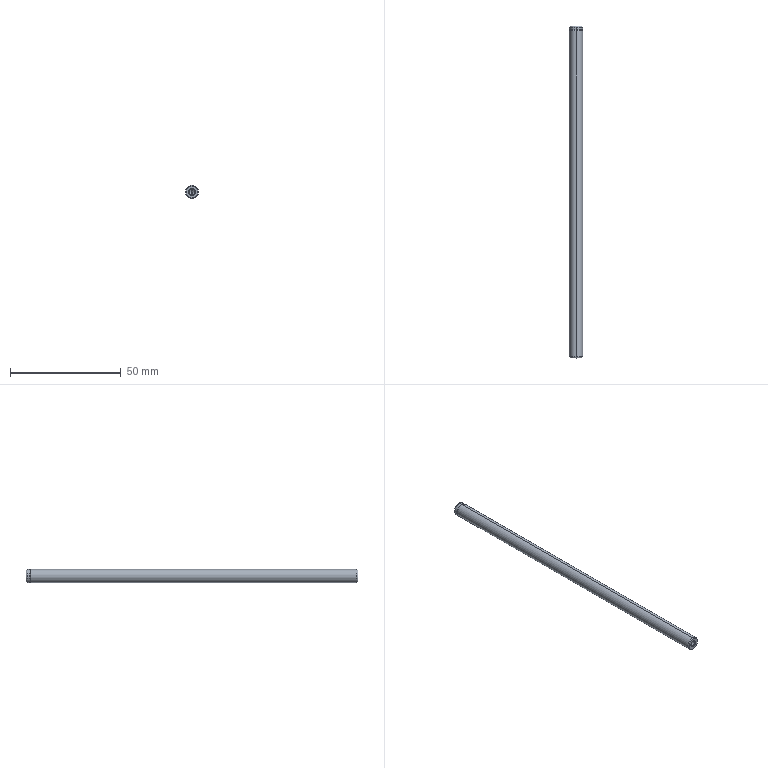Part | STEP file | MOP-150-1.step-29.STEP.STEP-2.STEP.STEP-277.STEP | 1 solid | 26 faces | box 6 x 150 x 6 mm | volume 4190 mm3 | cone 16 | cylinder 8 | plane 2 | commonest cylinder face diameters 2.5 x4 6 x4
STEP:
#1=CARTESIAN_POINT('',(0.,147.8,3.));
#2=VERTEX_POINT('',#1);
#3=CARTESIAN_POINT('',(0.,147.8,-3.));
#4=VERTEX_POINT('',#3);
#5=CARTESIAN_POINT('',(0.,147.8,0.));
#6=DIRECTION('',(0.,1.,0.));
#7=DIRECTION('',(0.,0.,-1.));
#8=AXIS2_PLACEMENT_3D('',#5,#6,#7);
#9=CIRCLE('',#8,3.);
#10=EDGE_CURVE('',#2,#4,#9,.T.);
#11=ORIENTED_EDGE('',*,*,#10,.F.);
#12=CARTESIAN_POINT('',(0.,0.5196,3.));
#13=VERTEX_POINT('',#12);
#14=CARTESIAN_POINT('',(0.,150.,3.));
#15=DIRECTION('',(0.,-1.,0.));
#16=VECTOR('',#15,1000.);
#17=LINE('',#14,#16);
#18=EDGE_CURVE('',#2,#13,#17,.T.);
#19=ORIENTED_EDGE('',*,*,#18,.T.);
#20=CARTESIAN_POINT('',(0.,0.5196,-3.));
#21=VERTEX_POINT('',#20);
#22=CARTESIAN_POINT('',(0.,0.5196,0.));
#23=DIRECTION('',(0.,1.,0.));
#24=DIRECTION('',(0.,0.,1.));
#25=AXIS2_PLACEMENT_3D('',#22,#23,#24);
#26=CIRCLE('',#25,3.);
#27=EDGE_CURVE('',#13,#21,#26,.T.);
#28=ORIENTED_EDGE('',*,*,#27,.T.);
#29=CARTESIAN_POINT('',(0.,150.,-3.));
#30=DIRECTION('',(0.,-1.,0.));
#31=VECTOR('',#30,1000.);
#32=LINE('',#29,#31);
#33=EDGE_CURVE('',#4,#21,#32,.T.);
#34=ORIENTED_EDGE('',*,*,#33,.F.);
#35=EDGE_LOOP('',(#11,#19,#28,#34));
#36=FACE_OUTER_BOUND('',#35,.T.);
#37=CARTESIAN_POINT('',(0.,150.,0.));
#38=DIRECTION('',(0.,-1.,0.));
#39=DIRECTION('',(0.,0.,-1.));
#40=AXIS2_PLACEMENT_3D('',#37,#38,#39);
#41=CYLINDRICAL_SURFACE('',#40,3.);
#42=ADVANCED_FACE('',(#36),#41,.T.);
#43=CARTESIAN_POINT('',(0.,0.,-2.7));
#44=VERTEX_POINT('',#43);
#45=CARTESIAN_POINT('',(0.,0.,2.7));
#46=VERTEX_POINT('',#45);
#47=CARTESIAN_POINT('',(0.,0.,0.));
#48=DIRECTION('',(0.,-1.,0.));
#49=DIRECTION('',(0.,0.,1.));
#50=AXIS2_PLACEMENT_3D('',#47,#48,#49);
#51=CIRCLE('',#50,2.7);
#52=EDGE_CURVE('',#44,#46,#51,.T.);
#53=ORIENTED_EDGE('',*,*,#52,.F.);
#54=CARTESIAN_POINT('',(0.,0.5196,-3.));
#55=DIRECTION('',(0.,0.866,-0.5));
#56=VECTOR('',#55,1000.);
#57=LINE('',#54,#56);
#58=EDGE_CURVE('',#44,#21,#57,.T.);
#59=ORIENTED_EDGE('',*,*,#58,.T.);
#60=ORIENTED_EDGE('',*,*,#27,.F.);
#61=CARTESIAN_POINT('',(0.,0.5196,3.));
#62=DIRECTION('',(0.,0.866,0.5));
#63=VECTOR('',#62,1000.);
#64=LINE('',#61,#63);
#65=EDGE_CURVE('',#46,#13,#64,.T.);
#66=ORIENTED_EDGE('',*,*,#65,.F.);
#67=EDGE_LOOP('',(#53,#59,#60,#66));
#68=FACE_OUTER_BOUND('',#67,.T.);
#69=CARTESIAN_POINT('',(0.,0.5196,0.));
#70=DIRECTION('',(0.,1.,0.));
#71=DIRECTION('',(0.,0.,1.));
#72=AXIS2_PLACEMENT_3D('',#69,#70,#71);
#73=CONICAL_SURFACE('',#72,3.,0.5236);
#74=ADVANCED_FACE('',(#68),#73,.T.);
#75=CARTESIAN_POINT('',(0.,0.3,1.25));
#76=VERTEX_POINT('',#75);
#77=CARTESIAN_POINT('',(0.,0.3,-1.25));
#78=VERTEX_POINT('',#77);
#79=CARTESIAN_POINT('',(0.,0.3,0.));
#80=DIRECTION('',(0.,-1.,0.));
#81=DIRECTION('',(0.,0.,1.));
#82=AXIS2_PLACEMENT_3D('',#79,#80,#81);
#83=CIRCLE('',#82,1.25);
#84=EDGE_CURVE('',#76,#78,#83,.T.);
#85=ORIENTED_EDGE('',*,*,#84,.F.);
#86=CARTESIAN_POINT('',(0.,0.,1.55));
#87=VERTEX_POINT('',#86);
#88=CARTESIAN_POINT('',(0.,0.3,1.25));
#89=DIRECTION('',(0.,-0.7071,0.7071));
#90=VECTOR('',#89,1000.);
#91=LINE('',#88,#90);
#92=EDGE_CURVE('',#76,#87,#91,.T.);
#93=ORIENTED_EDGE('',*,*,#92,.T.);
#94=CARTESIAN_POINT('',(0.,0.,-1.55));
#95=VERTEX_POINT('',#94);
#96=CARTESIAN_POINT('',(0.,0.,0.));
#97=DIRECTION('',(0.,1.,0.));
#98=DIRECTION('',(0.,0.,1.));
#99=AXIS2_PLACEMENT_3D('',#96,#97,#98);
#100=CIRCLE('',#99,1.55);
#101=EDGE_CURVE('',#95,#87,#100,.T.);
#102=ORIENTED_EDGE('',*,*,#101,.F.);
#103=CARTESIAN_POINT('',(0.,0.3,-1.25));
#104=DIRECTION('',(0.,-0.7071,-0.7071));
#105=VECTOR('',#104,1000.);
#106=LINE('',#103,#105);
#107=EDGE_CURVE('',#78,#95,#106,.T.);
#108=ORIENTED_EDGE('',*,*,#107,.F.);
#109=EDGE_LOOP('',(#85,#93,#102,#108));
#110=FACE_OUTER_BOUND('',#109,.T.);
#111=CARTESIAN_POINT('',(0.,0.3,0.));
#112=DIRECTION('',(0.,-1.,0.));
#113=DIRECTION('',(0.,0.,-1.));
#114=AXIS2_PLACEMENT_3D('',#111,#112,#113);
#115=CONICAL_SURFACE('',#114,1.25,0.7854);
#116=ADVANCED_FACE('',(#110),#115,.F.);
#117=CARTESIAN_POINT('',(0.,4.5,1.25));
#118=VERTEX_POINT('',#117);
#119=CARTESIAN_POINT('',(0.,4.5,-1.25));
#120=VERTEX_POINT('',#119);
#121=CARTESIAN_POINT('',(0.,4.5,0.));
#122=DIRECTION('',(0.,-1.,0.));
#123=DIRECTION('',(0.,0.,-1.));
#124=AXIS2_PLACEMENT_3D('',#121,#122,#123);
#125=CIRCLE('',#124,1.25);
#126=EDGE_CURVE('',#118,#120,#125,.T.);
#127=ORIENTED_EDGE('',*,*,#126,.F.);
#128=CARTESIAN_POINT('',(0.,0.,1.25));
#129=DIRECTION('',(0.,-1.,0.));
#130=VECTOR('',#129,1000.);
#131=LINE('',#128,#130);
#132=EDGE_CURVE('',#118,#76,#131,.T.);
#133=ORIENTED_EDGE('',*,*,#132,.T.);
#134=ORIENTED_EDGE('',*,*,#84,.T.);
#135=CARTESIAN_POINT('',(0.,0.,-1.25));
#136=DIRECTION('',(0.,-1.,0.));
#137=VECTOR('',#136,1000.);
#138=LINE('',#135,#137);
#139=EDGE_CURVE('',#120,#78,#138,.T.);
#140=ORIENTED_EDGE('',*,*,#139,.F.);
#141=EDGE_LOOP('',(#127,#133,#134,#140));
#142=FACE_OUTER_BOUND('',#141,.T.);
#143=CARTESIAN_POINT('',(0.,0.,0.));
#144=DIRECTION('',(0.,-1.,0.));
#145=DIRECTION('',(0.,0.,-1.));
#146=AXIS2_PLACEMENT_3D('',#143,#144,#145);
#147=CYLINDRICAL_SURFACE('',#146,1.25);
#148=ADVANCED_FACE('',(#142),#147,.F.);
#149=CARTESIAN_POINT('',(0.,5.251,0.));
#150=VERTEX_POINT('',#149);
#151=CARTESIAN_POINT('',(0.,4.5,-1.25));
#152=DIRECTION('',(0.,-0.515,-0.8572));
#153=VECTOR('',#152,1000.);
#154=LINE('',#151,#153);
#155=EDGE_CURVE('',#150,#120,#154,.T.);
#156=ORIENTED_EDGE('',*,*,#155,.F.);
#157=CARTESIAN_POINT('',(0.,4.5,1.25));
#158=DIRECTION('',(0.,-0.515,0.8572));
#159=VECTOR('',#158,1000.);
#160=LINE('',#157,#159);
#161=EDGE_CURVE('',#150,#118,#160,.T.);
#162=ORIENTED_EDGE('',*,*,#161,.T.);
#163=ORIENTED_EDGE('',*,*,#126,.T.);
#164=EDGE_LOOP('',(#156,#162,#163));
#165=FACE_OUTER_BOUND('',#164,.T.);
#166=CARTESIAN_POINT('',(0.,4.5,0.));
#167=DIRECTION('',(0.,-1.,0.));
#168=DIRECTION('',(0.,0.,-1.));
#169=AXIS2_PLACEMENT_3D('',#166,#167,#168);
#170=CONICAL_SURFACE('',#169,1.25,1.03);
#171=ADVANCED_FACE('',(#165),#170,.F.);
#172=CARTESIAN_POINT('',(0.,148.,-2.8));
#173=VERTEX_POINT('',#172);
#174=CARTESIAN_POINT('',(0.,148.,2.8));
#175=VERTEX_POINT('',#174);
#176=CARTESIAN_POINT('',(0.,148.,0.));
#177=DIRECTION('',(0.,-1.,0.));
#178=DIRECTION('',(0.,0.,-1.));
#179=AXIS2_PLACEMENT_3D('',#176,#177,#178);
#180=CIRCLE('',#179,2.8);
#181=EDGE_CURVE('',#173,#175,#180,.T.);
#182=ORIENTED_EDGE('',*,*,#181,.T.);
#183=CARTESIAN_POINT('',(0.,2.194,148.606));
#184=DIRECTION('',(0.,-0.7071,0.7071));
#185=VECTOR('',#184,1000.);
#186=LINE('',#183,#185);
#187=EDGE_CURVE('',#175,#2,#186,.T.);
#188=ORIENTED_EDGE('',*,*,#187,.T.);
#189=ORIENTED_EDGE('',*,*,#10,.T.);
#190=CARTESIAN_POINT('',(0.,2.194,-148.606));
#191=DIRECTION('',(0.,-0.7071,-0.7071));
#192=VECTOR('',#191,1000.);
#193=LINE('',#190,#192);
#194=EDGE_CURVE('',#173,#4,#193,.T.);
#195=ORIENTED_EDGE('',*,*,#194,.F.);
#196=EDGE_LOOP('',(#182,#188,#189,#195));
#197=FACE_OUTER_BOUND('',#196,.T.);
#198=CARTESIAN_POINT('',(0.,2.194,0.));
#199=DIRECTION('',(0.,-1.,0.));
#200=DIRECTION('',(0.,0.,-1.));
#201=AXIS2_PLACEMENT_3D('',#198,#199,#200);
#202=CONICAL_SURFACE('',#201,148.606,0.7854);
#203=ADVANCED_FACE('',(#197),#202,.T.);
#204=ORIENTED_EDGE('',*,*,#181,.F.);
#205=CARTESIAN_POINT('',(0.,148.2,-3.));
#206=VERTEX_POINT('',#205);
#207=CARTESIAN_POINT('',(0.,148.,-2.8));
#208=DIRECTION('',(0.,0.7071,-0.7071));
#209=VECTOR('',#208,1000.);
#210=LINE('',#207,#209);
#211=EDGE_CURVE('',#173,#206,#210,.T.);
#212=ORIENTED_EDGE('',*,*,#211,.T.);
#213=CARTESIAN_POINT('',(0.,148.2,3.));
#214=VERTEX_POINT('',#213);
#215=CARTESIAN_POINT('',(0.,148.2,0.));
#216=DIRECTION('',(0.,-1.,0.));
#217=DIRECTION('',(0.,0.,1.));
#218=AXIS2_PLACEMENT_3D('',#215,#216,#217);
#219=CIRCLE('',#218,3.);
#220=EDGE_CURVE('',#206,#214,#219,.T.);
#221=ORIENTED_EDGE('',*,*,#220,.T.);
#222=CARTESIAN_POINT('',(0.,148.,2.8));
#223=DIRECTION('',(0.,0.7071,0.7071));
#224=VECTOR('',#223,1000.);
#225=LINE('',#222,#224);
#226=EDGE_CURVE('',#175,#214,#225,.T.);
#227=ORIENTED_EDGE('',*,*,#226,.F.);
#228=EDGE_LOOP('',(#204,#212,#221,#227));
#229=FACE_OUTER_BOUND('',#228,.T.);
#230=CARTESIAN_POINT('',(0.,148.,0.));
#231=DIRECTION('',(0.,1.,0.));
#232=DIRECTION('',(0.,0.,1.));
#233=AXIS2_PLACEMENT_3D('',#230,#231,#232);
#234=CONICAL_SURFACE('',#233,2.8,0.7854);
#235=ADVANCED_FACE('',(#229),#234,.T.);
#236=CARTESIAN_POINT('',(0.,149.7,-1.25));
#237=VERTEX_POINT('',#236);
#238=CARTESIAN_POINT('',(0.,149.7,1.25));
#239=VERTEX_POINT('',#238);
#240=CARTESIAN_POINT('',(0.,149.7,0.));
#241=DIRECTION('',(0.,1.,0.));
#242=DIRECTION('',(0.,0.,1.));
#243=AXIS2_PLACEMENT_3D('',#240,#241,#242);
#244=CIRCLE('',#243,1.25);
#245=EDGE_CURVE('',#237,#239,#244,.T.);
#246=ORIENTED_EDGE('',*,*,#245,.F.);
#247=CARTESIAN_POINT('',(0.,150.,-1.55));
#248=VERTEX_POINT('',#247);
#249=CARTESIAN_POINT('',(0.,149.7,-1.25));
#250=DIRECTION('',(0.,0.7071,-0.7071));
#251=VECTOR('',#250,1000.);
#252=LINE('',#249,#251);
#253=EDGE_CURVE('',#237,#248,#252,.T.);
#254=ORIENTED_EDGE('',*,*,#253,.T.);
#255=CARTESIAN_POINT('',(0.,150.,1.55));
#256=VERTEX_POINT('',#255);
#257=CARTESIAN_POINT('',(0.,150.,0.));
#258=DIRECTION('',(0.,-1.,0.));
#259=DIRECTION('',(0.,0.,1.));
#260=AXIS2_PLACEMENT_3D('',#257,#258,#259);
#261=CIRCLE('',#260,1.55);
#262=EDGE_CURVE('',#256,#248,#261,.T.);
#263=ORIENTED_EDGE('',*,*,#262,.F.);
#264=CARTESIAN_POINT('',(0.,149.7,1.25));
#265=DIRECTION('',(0.,0.7071,0.7071));
#266=VECTOR('',#265,1000.);
#267=LINE('',#264,#266);
#268=EDGE_CURVE('',#239,#256,#267,.T.);
#269=ORIENTED_EDGE('',*,*,#268,.F.);
#270=EDGE_LOOP('',(#246,#254,#263,#269));
#271=FACE_OUTER_BOUND('',#270,.T.);
#272=CARTESIAN_POINT('',(0.,149.7,0.));
#273=DIRECTION('',(0.,1.,0.));
#274=DIRECTION('',(0.,0.,1.));
#275=AXIS2_PLACEMENT_3D('',#272,#273,#274);
#276=CONICAL_SURFACE('',#275,1.25,0.7854);
#277=ADVANCED_FACE('',(#271),#276,.F.);
#278=CARTESIAN_POINT('',(0.,150.,2.7));
#279=VERTEX_POINT('',#278);
#280=CARTESIAN_POINT('',(0.,150.,-2.7));
#281=VERTEX_POINT('',#280);
#282=CARTESIAN_POINT('',(0.,150.,0.));
#283=DIRECTION('',(0.,1.,0.));
#284=DIRECTION('',(0.,0.,1.));
#285=AXIS2_PLACEMENT_3D('',#282,#283,#284);
#286=CIRCLE('',#285,2.7);
#287=EDGE_CURVE('',#279,#281,#286,.T.);
#288=ORIENTED_EDGE('',*,*,#287,.F.);
#289=CARTESIAN_POINT('',(0.,149.48,3.));
#290=VERTEX_POINT('',#289);
#291=CARTESIAN_POINT('',(0.,150.,2.7));
#292=DIRECTION('',(0.,-0.866,0.5));
#293=VECTOR('',#292,1000.);
#294=LINE('',#291,#293);
#295=EDGE_CURVE('',#279,#290,#294,.T.);
#296=ORIENTED_EDGE('',*,*,#295,.T.);
#297=CARTESIAN_POINT('',(0.,149.48,-3.));
#298=VERTEX_POINT('',#297);
#299=CARTESIAN_POINT('',(0.,149.48,0.));
#300=DIRECTION('',(0.,-1.,0.));
#301=DIRECTION('',(0.,0.,1.));
#302=AXIS2_PLACEMENT_3D('',#299,#300,#301);
#303=CIRCLE('',#302,3.);
#304=EDGE_CURVE('',#298,#290,#303,.T.);
#305=ORIENTED_EDGE('',*,*,#304,.F.);
#306=CARTESIAN_POINT('',(0.,150.,-2.7));
#307=DIRECTION('',(0.,-0.866,-0.5));
#308=VECTOR('',#307,1000.);
#309=LINE('',#306,#308);
#310=EDGE_CURVE('',#281,#298,#309,.T.);
#311=ORIENTED_EDGE('',*,*,#310,.F.);
#312=EDGE_LOOP('',(#288,#296,#305,#311));
#313=FACE_OUTER_BOUND('',#312,.T.);
#314=CARTESIAN_POINT('',(0.,150.,0.));
#315=DIRECTION('',(0.,-1.,0.));
#316=DIRECTION('',(0.,0.,-1.));
#317=AXIS2_PLACEMENT_3D('',#314,#315,#316);
#318=CONICAL_SURFACE('',#317,2.7,0.5236);
#319=ADVANCED_FACE('',(#313),#318,.T.);
#320=CARTESIAN_POINT('',(0.,145.5,-1.25));
#321=VERTEX_POINT('',#320);
#322=CARTESIAN_POINT('',(0.,145.5,1.25));
#323=VERTEX_POINT('',#322);
#324=CARTESIAN_POINT('',(0.,145.5,0.));
#325=DIRECTION('',(0.,1.,0.));
#326=DIRECTION('',(0.,0.,1.));
#327=AXIS2_PLACEMENT_3D('',#324,#325,#326);
#328=CIRCLE('',#327,1.25);
#329=EDGE_CURVE('',#321,#323,#328,.T.);
#330=ORIENTED_EDGE('',*,*,#329,.F.);
#331=CARTESIAN_POINT('',(0.,150.,-1.25));
#332=DIRECTION('',(0.,1.,0.));
#333=VECTOR('',#332,1000.);
#334=LINE('',#331,#333);
#335=EDGE_CURVE('',#321,#237,#334,.T.);
#336=ORIENTED_EDGE('',*,*,#335,.T.);
#337=ORIENTED_EDGE('',*,*,#245,.T.);
#338=CARTESIAN_POINT('',(0.,150.,1.25));
#339=DIRECTION('',(0.,1.,0.));
#340=VECTOR('',#339,1000.);
#341=LINE('',#338,#340);
#342=EDGE_CURVE('',#323,#239,#341,.T.);
#343=ORIENTED_EDGE('',*,*,#342,.F.);
#344=EDGE_LOOP('',(#330,#336,#337,#343));
#345=FACE_OUTER_BOUND('',#344,.T.);
#346=CARTESIAN_POINT('',(0.,150.,0.));
#347=DIRECTION('',(0.,1.,0.));
#348=DIRECTION('',(0.,0.,1.));
#349=AXIS2_PLACEMENT_3D('',#346,#347,#348);
#350=CYLINDRICAL_SURFACE('',#349,1.25);
#351=ADVANCED_FACE('',(#345),#350,.F.);
#352=CARTESIAN_POINT('',(0.,144.749,0.));
#353=VERTEX_POINT('',#352);
#354=CARTESIAN_POINT('',(0.,145.5,1.25));
#355=DIRECTION('',(0.,0.515,0.8572));
#356=VECTOR('',#355,1000.);
#357=LINE('',#354,#356);
#358=EDGE_CURVE('',#353,#323,#357,.T.);
#359=ORIENTED_EDGE('',*,*,#358,.F.);
#360=CARTESIAN_POINT('',(0.,145.5,-1.25));
#361=DIRECTION('',(0.,0.515,-0.8572));
#362=VECTOR('',#361,1000.);
#363=LINE('',#360,#362);
#364=EDGE_CURVE('',#353,#321,#363,.T.);
#365=ORIENTED_EDGE('',*,*,#364,.T.);
#366=ORIENTED_EDGE('',*,*,#329,.T.);
#367=EDGE_LOOP('',(#359,#365,#366));
#368=FACE_OUTER_BOUND('',#367,.T.);
#369=CARTESIAN_POINT('',(0.,145.5,0.));
#370=DIRECTION('',(0.,1.,0.));
#371=DIRECTION('',(0.,0.,1.));
#372=AXIS2_PLACEMENT_3D('',#369,#370,#371);
#373=CONICAL_SURFACE('',#372,1.25,1.03);
#374=ADVANCED_FACE('',(#368),#373,.F.);
#375=ORIENTED_EDGE('',*,*,#304,.T.);
#376=CARTESIAN_POINT('',(0.,150.,3.));
#377=DIRECTION('',(0.,-1.,0.));
#378=VECTOR('',#377,1000.);
#379=LINE('',#376,#378);
#380=EDGE_CURVE('',#290,#214,#379,.T.);
#381=ORIENTED_EDGE('',*,*,#380,.T.);
#382=ORIENTED_EDGE('',*,*,#220,.F.);
#383=CARTESIAN_POINT('',(0.,150.,-3.));
#384=DIRECTION('',(0.,-1.,0.));
#385=VECTOR('',#384,1000.);
#386=LINE('',#383,#385);
#387=EDGE_CURVE('',#298,#206,#386,.T.);
#388=ORIENTED_EDGE('',*,*,#387,.F.);
#389=EDGE_LOOP('',(#375,#381,#382,#388));
#390=FACE_OUTER_BOUND('',#389,.T.);
#391=CARTESIAN_POINT('',(0.,150.,0.));
#392=DIRECTION('',(0.,-1.,0.));
#393=DIRECTION('',(0.,0.,-1.));
#394=AXIS2_PLACEMENT_3D('',#391,#392,#393);
#395=CYLINDRICAL_SURFACE('',#394,3.);
#396=ADVANCED_FACE('',(#390),#395,.T.);
#397=ORIENTED_EDGE('',*,*,#380,.F.);
#398=CARTESIAN_POINT('',(0.,149.48,0.));
#399=DIRECTION('',(0.,-1.,0.));
#400=DIRECTION('',(0.,0.,1.));
#401=AXIS2_PLACEMENT_3D('',#398,#399,#400);
#402=CIRCLE('',#401,3.);
#403=EDGE_CURVE('',#290,#298,#402,.T.);
#404=ORIENTED_EDGE('',*,*,#403,.T.);
#405=ORIENTED_EDGE('',*,*,#387,.T.);
#406=CARTESIAN_POINT('',(0.,148.2,0.));
#407=DIRECTION('',(0.,-1.,0.));
#408=DIRECTION('',(0.,0.,1.));
#409=AXIS2_PLACEMENT_3D('',#406,#407,#408);
#410=CIRCLE('',#409,3.);
#411=EDGE_CURVE('',#214,#206,#410,.T.);
#412=ORIENTED_EDGE('',*,*,#411,.F.);
#413=EDGE_LOOP('',(#397,#404,#405,#412));
#414=FACE_OUTER_BOUND('',#413,.T.);
#415=CARTESIAN_POINT('',(0.,150.,0.));
#416=DIRECTION('',(0.,-1.,0.));
#417=DIRECTION('',(0.,0.,-1.));
#418=AXIS2_PLACEMENT_3D('',#415,#416,#417);
#419=CYLINDRICAL_SURFACE('',#418,3.);
#420=ADVANCED_FACE('',(#414),#419,.T.);
#421=ORIENTED_EDGE('',*,*,#262,.T.);
#422=CARTESIAN_POINT('',(0.,150.,0.));
#423=DIRECTION('',(0.,-1.,0.));
#424=DIRECTION('',(0.,0.,1.));
#425=AXIS2_PLACEMENT_3D('',#422,#423,#424);
#426=CIRCLE('',#425,1.55);
#427=EDGE_CURVE('',#248,#256,#426,.T.);
#428=ORIENTED_EDGE('',*,*,#427,.T.);
#429=EDGE_LOOP('',(#421,#428));
#430=FACE_BOUND('',#429,.T.);
#431=CARTESIAN_POINT('',(0.,150.,0.));
#432=DIRECTION('',(0.,1.,0.));
#433=DIRECTION('',(0.,0.,1.));
#434=AXIS2_PLACEMENT_3D('',#431,#432,#433);
#435=CIRCLE('',#434,2.7);
#436=EDGE_CURVE('',#281,#279,#435,.T.);
#437=ORIENTED_EDGE('',*,*,#436,.T.);
#438=ORIENTED_EDGE('',*,*,#287,.T.);
#439=EDGE_LOOP('',(#437,#438));
#440=FACE_OUTER_BOUND('',#439,.T.);
#441=CARTESIAN_POINT('',(0.,150.,0.));
#442=DIRECTION('',(0.,1.,0.));
#443=DIRECTION('',(1.,0.,0.));
#444=AXIS2_PLACEMENT_3D('',#441,#442,#443);
#445=PLANE('',#444);
#446=ADVANCED_FACE('',(#430,#440),#445,.T.);
#447=ORIENTED_EDGE('',*,*,#364,.F.);
#448=ORIENTED_EDGE('',*,*,#358,.T.);
#449=CARTESIAN_POINT('',(0.,145.5,0.));
#450=DIRECTION('',(0.,1.,0.));
#451=DIRECTION('',(0.,0.,1.));
#452=AXIS2_PLACEMENT_3D('',#449,#450,#451);
#453=CIRCLE('',#452,1.25);
#454=EDGE_CURVE('',#323,#321,#453,.T.);
#455=ORIENTED_EDGE('',*,*,#454,.T.);
#456=EDGE_LOOP('',(#447,#448,#455));
#457=FACE_OUTER_BOUND('',#456,.T.);
#458=CARTESIAN_POINT('',(0.,145.5,0.));
#459=DIRECTION('',(0.,1.,0.));
#460=DIRECTION('',(0.,0.,1.));
#461=AXIS2_PLACEMENT_3D('',#458,#459,#460);
#462=CONICAL_SURFACE('',#461,1.25,1.03);
#463=ADVANCED_FACE('',(#457),#462,.F.);
#464=ORIENTED_EDGE('',*,*,#335,.F.);
#465=ORIENTED_EDGE('',*,*,#454,.F.);
#466=ORIENTED_EDGE('',*,*,#342,.T.);
#467=CARTESIAN_POINT('',(0.,149.7,0.));
#468=DIRECTION('',(0.,1.,0.));
#469=DIRECTION('',(0.,0.,1.));
#470=AXIS2_PLACEMENT_3D('',#467,#468,#469);
#471=CIRCLE('',#470,1.25);
#472=EDGE_CURVE('',#239,#237,#471,.T.);
#473=ORIENTED_EDGE('',*,*,#472,.T.);
#474=EDGE_LOOP('',(#464,#465,#466,#473));
#475=FACE_OUTER_BOUND('',#474,.T.);
#476=CARTESIAN_POINT('',(0.,150.,0.));
#477=DIRECTION('',(0.,1.,0.));
#478=DIRECTION('',(0.,0.,1.));
#479=AXIS2_PLACEMENT_3D('',#476,#477,#478);
#480=CYLINDRICAL_SURFACE('',#479,1.25);
#481=ADVANCED_FACE('',(#475),#480,.F.);
#482=ORIENTED_EDGE('',*,*,#295,.F.);
#483=ORIENTED_EDGE('',*,*,#436,.F.);
#484=ORIENTED_EDGE('',*,*,#310,.T.);
#485=ORIENTED_EDGE('',*,*,#403,.F.);
#486=EDGE_LOOP('',(#482,#483,#484,#485));
#487=FACE_OUTER_BOUND('',#486,.T.);
#488=CARTESIAN_POINT('',(0.,150.,0.));
#489=DIRECTION('',(0.,-1.,0.));
#490=DIRECTION('',(0.,0.,-1.));
#491=AXIS2_PLACEMENT_3D('',#488,#489,#490);
#492=CONICAL_SURFACE('',#491,2.7,0.5236);
#493=ADVANCED_FACE('',(#487),#492,.T.);
#494=ORIENTED_EDGE('',*,*,#253,.F.);
#495=ORIENTED_EDGE('',*,*,#472,.F.);
#496=ORIENTED_EDGE('',*,*,#268,.T.);
#497=ORIENTED_EDGE('',*,*,#427,.F.);
#498=EDGE_LOOP('',(#494,#495,#496,#497));
#499=FACE_OUTER_BOUND('',#498,.T.);
#500=CARTESIAN_POINT('',(0.,149.7,0.));
#501=DIRECTION('',(0.,1.,0.));
#502=DIRECTION('',(0.,0.,1.));
#503=AXIS2_PLACEMENT_3D('',#500,#501,#502);
#504=CONICAL_SURFACE('',#503,1.25,0.7854);
#505=ADVANCED_FACE('',(#499),#504,.F.);
#506=ORIENTED_EDGE('',*,*,#211,.F.);
#507=CARTESIAN_POINT('',(0.,148.,0.));
#508=DIRECTION('',(0.,-1.,0.));
#509=DIRECTION('',(0.,0.,-1.));
#510=AXIS2_PLACEMENT_3D('',#507,#508,#509);
#511=CIRCLE('',#510,2.8);
#512=EDGE_CURVE('',#175,#173,#511,.T.);
#513=ORIENTED_EDGE('',*,*,#512,.F.);
#514=ORIENTED_EDGE('',*,*,#226,.T.);
#515=ORIENTED_EDGE('',*,*,#411,.T.);
#516=EDGE_LOOP('',(#506,#513,#514,#515));
#517=FACE_OUTER_BOUND('',#516,.T.);
#518=CARTESIAN_POINT('',(0.,148.,0.));
#519=DIRECTION('',(0.,1.,0.));
#520=DIRECTION('',(0.,0.,1.));
#521=AXIS2_PLACEMENT_3D('',#518,#519,#520);
#522=CONICAL_SURFACE('',#521,2.8,0.7854);
#523=ADVANCED_FACE('',(#517),#522,.T.);
#524=ORIENTED_EDGE('',*,*,#187,.F.);
#525=ORIENTED_EDGE('',*,*,#512,.T.);
#526=ORIENTED_EDGE('',*,*,#194,.T.);
#527=CARTESIAN_POINT('',(0.,147.8,0.));
#528=DIRECTION('',(0.,1.,0.));
#529=DIRECTION('',(0.,0.,-1.));
#530=AXIS2_PLACEMENT_3D('',#527,#528,#529);
#531=CIRCLE('',#530,3.);
#532=EDGE_CURVE('',#4,#2,#531,.T.);
#533=ORIENTED_EDGE('',*,*,#532,.T.);
#534=EDGE_LOOP('',(#524,#525,#526,#533));
#535=FACE_OUTER_BOUND('',#534,.T.);
#536=CARTESIAN_POINT('',(0.,2.194,0.));
#537=DIRECTION('',(0.,-1.,0.));
#538=DIRECTION('',(0.,0.,-1.));
#539=AXIS2_PLACEMENT_3D('',#536,#537,#538);
#540=CONICAL_SURFACE('',#539,148.606,0.7854);
#541=ADVANCED_FACE('',(#535),#540,.T.);
#542=ORIENTED_EDGE('',*,*,#161,.F.);
#543=ORIENTED_EDGE('',*,*,#155,.T.);
#544=CARTESIAN_POINT('',(0.,4.5,0.));
#545=DIRECTION('',(0.,-1.,0.));
#546=DIRECTION('',(0.,0.,-1.));
#547=AXIS2_PLACEMENT_3D('',#544,#545,#546);
#548=CIRCLE('',#547,1.25);
#549=EDGE_CURVE('',#120,#118,#548,.T.);
#550=ORIENTED_EDGE('',*,*,#549,.T.);
#551=EDGE_LOOP('',(#542,#543,#550));
#552=FACE_OUTER_BOUND('',#551,.T.);
#553=CARTESIAN_POINT('',(0.,4.5,0.));
#554=DIRECTION('',(0.,-1.,0.));
#555=DIRECTION('',(0.,0.,-1.));
#556=AXIS2_PLACEMENT_3D('',#553,#554,#555);
#557=CONICAL_SURFACE('',#556,1.25,1.03);
#558=ADVANCED_FACE('',(#552),#557,.F.);
#559=ORIENTED_EDGE('',*,*,#132,.F.);
#560=ORIENTED_EDGE('',*,*,#549,.F.);
#561=ORIENTED_EDGE('',*,*,#139,.T.);
#562=CARTESIAN_POINT('',(0.,0.3,0.));
#563=DIRECTION('',(0.,-1.,0.));
#564=DIRECTION('',(0.,0.,1.));
#565=AXIS2_PLACEMENT_3D('',#562,#563,#564);
#566=CIRCLE('',#565,1.25);
#567=EDGE_CURVE('',#78,#76,#566,.T.);
#568=ORIENTED_EDGE('',*,*,#567,.T.);
#569=EDGE_LOOP('',(#559,#560,#561,#568));
#570=FACE_OUTER_BOUND('',#569,.T.);
#571=CARTESIAN_POINT('',(0.,0.,0.));
#572=DIRECTION('',(0.,-1.,0.));
#573=DIRECTION('',(0.,0.,-1.));
#574=AXIS2_PLACEMENT_3D('',#571,#572,#573);
#575=CYLINDRICAL_SURFACE('',#574,1.25);
#576=ADVANCED_FACE('',(#570),#575,.F.);
#577=ORIENTED_EDGE('',*,*,#92,.F.);
#578=ORIENTED_EDGE('',*,*,#567,.F.);
#579=ORIENTED_EDGE('',*,*,#107,.T.);
#580=CARTESIAN_POINT('',(0.,0.,0.));
#581=DIRECTION('',(0.,1.,0.));
#582=DIRECTION('',(0.,0.,1.));
#583=AXIS2_PLACEMENT_3D('',#580,#581,#582);
#584=CIRCLE('',#583,1.55);
#585=EDGE_CURVE('',#87,#95,#584,.T.);
#586=ORIENTED_EDGE('',*,*,#585,.F.);
#587=EDGE_LOOP('',(#577,#578,#579,#586));
#588=FACE_OUTER_BOUND('',#587,.T.);
#589=CARTESIAN_POINT('',(0.,0.3,0.));
#590=DIRECTION('',(0.,-1.,0.));
#591=DIRECTION('',(0.,0.,-1.));
#592=AXIS2_PLACEMENT_3D('',#589,#590,#591);
#593=CONICAL_SURFACE('',#592,1.25,0.7854);
#594=ADVANCED_FACE('',(#588),#593,.F.);
#595=ORIENTED_EDGE('',*,*,#101,.T.);
#596=ORIENTED_EDGE('',*,*,#585,.T.);
#597=EDGE_LOOP('',(#595,#596));
#598=FACE_BOUND('',#597,.T.);
#599=CARTESIAN_POINT('',(0.,0.,0.));
#600=DIRECTION('',(0.,-1.,0.));
#601=DIRECTION('',(0.,0.,1.));
#602=AXIS2_PLACEMENT_3D('',#599,#600,#601);
#603=CIRCLE('',#602,2.7);
#604=EDGE_CURVE('',#46,#44,#603,.T.);
#605=ORIENTED_EDGE('',*,*,#604,.T.);
#606=ORIENTED_EDGE('',*,*,#52,.T.);
#607=EDGE_LOOP('',(#605,#606));
#608=FACE_OUTER_BOUND('',#607,.T.);
#609=CARTESIAN_POINT('',(0.,0.,0.));
#610=DIRECTION('',(0.,1.,0.));
#611=DIRECTION('',(1.,0.,0.));
#612=AXIS2_PLACEMENT_3D('',#609,#610,#611);
#613=PLANE('',#612);
#614=ADVANCED_FACE('',(#598,#608),#613,.F.);
#615=ORIENTED_EDGE('',*,*,#58,.F.);
#616=ORIENTED_EDGE('',*,*,#604,.F.);
#617=ORIENTED_EDGE('',*,*,#65,.T.);
#618=CARTESIAN_POINT('',(0.,0.5196,0.));
#619=DIRECTION('',(0.,1.,0.));
#620=DIRECTION('',(0.,0.,1.));
#621=AXIS2_PLACEMENT_3D('',#618,#619,#620);
#622=CIRCLE('',#621,3.);
#623=EDGE_CURVE('',#21,#13,#622,.T.);
#624=ORIENTED_EDGE('',*,*,#623,.F.);
#625=EDGE_LOOP('',(#615,#616,#617,#624));
#626=FACE_OUTER_BOUND('',#625,.T.);
#627=CARTESIAN_POINT('',(0.,0.5196,0.));
#628=DIRECTION('',(0.,1.,0.));
#629=DIRECTION('',(0.,0.,1.));
#630=AXIS2_PLACEMENT_3D('',#627,#628,#629);
#631=CONICAL_SURFACE('',#630,3.,0.5236);
#632=ADVANCED_FACE('',(#626),#631,.T.);
#633=ORIENTED_EDGE('',*,*,#18,.F.);
#634=ORIENTED_EDGE('',*,*,#532,.F.);
#635=ORIENTED_EDGE('',*,*,#33,.T.);
#636=ORIENTED_EDGE('',*,*,#623,.T.);
#637=EDGE_LOOP('',(#633,#634,#635,#636));
#638=FACE_OUTER_BOUND('',#637,.T.);
#639=CARTESIAN_POINT('',(0.,150.,0.));
#640=DIRECTION('',(0.,-1.,0.));
#641=DIRECTION('',(0.,0.,-1.));
#642=AXIS2_PLACEMENT_3D('',#639,#640,#641);
#643=CYLINDRICAL_SURFACE('',#642,3.);
#644=ADVANCED_FACE('',(#638),#643,.T.);
#645=CLOSED_SHELL('',(#42,#74,#116,#148,#171,#203,#235,#277,#319,#351,#374,#396,#420,#446,#463,#481,#493,#505,#523,#541,#558,#576,#594,#614,#632,#644));
#646=MANIFOLD_SOLID_BREP('',#645);
#647=CARTESIAN_POINT('',(0.,0.,0.));
#648=DIRECTION('',(0.,0.,1.));
#649=DIRECTION('',(1.,0.,0.));
#650=AXIS2_PLACEMENT_3D('',#647,#648,#649);
#651=(LENGTH_UNIT()NAMED_UNIT(*)SI_UNIT(.MILLI.,.METRE.));
#652=UNCERTAINTY_MEASURE_WITH_UNIT(LENGTH_MEASURE(0.00001),#651,'','');
#653=(NAMED_UNIT(*)PLANE_ANGLE_UNIT()SI_UNIT($,.RADIAN.));
#654=(NAMED_UNIT(*)SI_UNIT($,.STERADIAN.)SOLID_ANGLE_UNIT());
#655=(GEOMETRIC_REPRESENTATION_CONTEXT(3)GLOBAL_UNCERTAINTY_ASSIGNED_CONTEXT((#652))GLOBAL_UNIT_ASSIGNED_CONTEXT((#651,#653,#654))REPRESENTATION_CONTEXT('',''));
#656=ADVANCED_BREP_SHAPE_REPRESENTATION('',(#646,#650),#655);